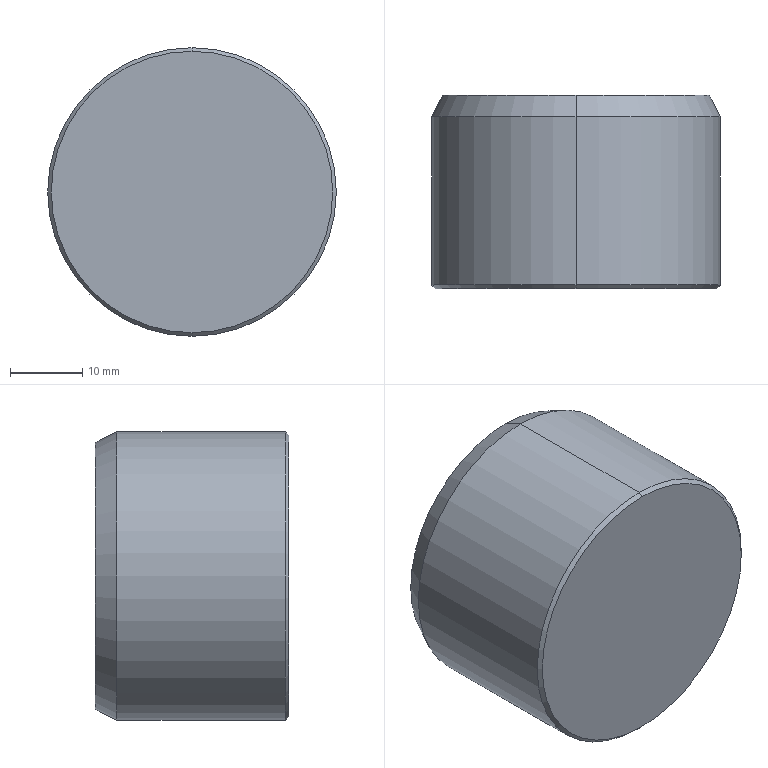Part | SolidWorks | features Chamfer 2, Revolution 1 | 1 solid | 8 faces | box 40 x 26.8 x 40 mm | volume 33387 mm3 | cone 4 | cylinder 2 | plane 2 | commonest cylinder face diameters 40 x2
STEP:
#1=CARTESIAN_POINT('',(0.,-13.4,-19.5));
#2=VERTEX_POINT('',#1);
#3=CARTESIAN_POINT('',(0.,-13.4,19.5));
#4=VERTEX_POINT('',#3);
#5=CARTESIAN_POINT('',(0.,-13.4,0.));
#6=DIRECTION('',(0.,-1.,0.));
#7=DIRECTION('',(0.,0.,-1.));
#8=AXIS2_PLACEMENT_3D('',#5,#6,#7);
#9=CIRCLE('',#8,19.5);
#10=EDGE_CURVE('',#2,#4,#9,.T.);
#11=ORIENTED_EDGE('',*,*,#10,.F.);
#12=CARTESIAN_POINT('',(0.,-12.9,-20.));
#13=VERTEX_POINT('',#12);
#14=CARTESIAN_POINT('',(0.,-13.4,-19.5));
#15=DIRECTION('',(0.,0.7071,-0.7071));
#16=VECTOR('',#15,1000.);
#17=LINE('',#14,#16);
#18=EDGE_CURVE('',#2,#13,#17,.T.);
#19=ORIENTED_EDGE('',*,*,#18,.T.);
#20=CARTESIAN_POINT('',(0.,-12.9,20.));
#21=VERTEX_POINT('',#20);
#22=CARTESIAN_POINT('',(0.,-12.9,0.));
#23=DIRECTION('',(0.,1.,0.));
#24=DIRECTION('',(0.,0.,-1.));
#25=AXIS2_PLACEMENT_3D('',#22,#23,#24);
#26=CIRCLE('',#25,20.);
#27=EDGE_CURVE('',#21,#13,#26,.T.);
#28=ORIENTED_EDGE('',*,*,#27,.F.);
#29=CARTESIAN_POINT('',(0.,-13.4,19.5));
#30=DIRECTION('',(0.,0.7071,0.7071));
#31=VECTOR('',#30,1000.);
#32=LINE('',#29,#31);
#33=EDGE_CURVE('',#4,#21,#32,.T.);
#34=ORIENTED_EDGE('',*,*,#33,.F.);
#35=EDGE_LOOP('',(#11,#19,#28,#34));
#36=FACE_OUTER_BOUND('',#35,.T.);
#37=CARTESIAN_POINT('',(0.,-13.4,0.));
#38=DIRECTION('',(0.,1.,0.));
#39=DIRECTION('',(0.,0.,1.));
#40=AXIS2_PLACEMENT_3D('',#37,#38,#39);
#41=CONICAL_SURFACE('',#40,19.5,0.7854);
#42=ADVANCED_FACE('',(#36),#41,.T.);
#43=CARTESIAN_POINT('',(0.,13.4,18.5));
#44=VERTEX_POINT('',#43);
#45=CARTESIAN_POINT('',(0.,13.4,-18.5));
#46=VERTEX_POINT('',#45);
#47=CARTESIAN_POINT('',(0.,13.4,0.));
#48=DIRECTION('',(0.,1.,0.));
#49=DIRECTION('',(0.,0.,1.));
#50=AXIS2_PLACEMENT_3D('',#47,#48,#49);
#51=CIRCLE('',#50,18.5);
#52=EDGE_CURVE('',#44,#46,#51,.T.);
#53=ORIENTED_EDGE('',*,*,#52,.F.);
#54=CARTESIAN_POINT('',(0.,10.4,20.));
#55=VERTEX_POINT('',#54);
#56=CARTESIAN_POINT('',(0.,10.4,20.));
#57=DIRECTION('',(0.,-0.8944,0.4472));
#58=VECTOR('',#57,1000.);
#59=LINE('',#56,#58);
#60=EDGE_CURVE('',#44,#55,#59,.T.);
#61=ORIENTED_EDGE('',*,*,#60,.T.);
#62=CARTESIAN_POINT('',(0.,10.4,-20.));
#63=VERTEX_POINT('',#62);
#64=CARTESIAN_POINT('',(0.,10.4,0.));
#65=DIRECTION('',(0.,-1.,0.));
#66=DIRECTION('',(0.,0.,1.));
#67=AXIS2_PLACEMENT_3D('',#64,#65,#66);
#68=CIRCLE('',#67,20.);
#69=EDGE_CURVE('',#63,#55,#68,.T.);
#70=ORIENTED_EDGE('',*,*,#69,.F.);
#71=CARTESIAN_POINT('',(0.,10.4,-20.));
#72=DIRECTION('',(0.,-0.8944,-0.4472));
#73=VECTOR('',#72,1000.);
#74=LINE('',#71,#73);
#75=EDGE_CURVE('',#46,#63,#74,.T.);
#76=ORIENTED_EDGE('',*,*,#75,.F.);
#77=EDGE_LOOP('',(#53,#61,#70,#76));
#78=FACE_OUTER_BOUND('',#77,.T.);
#79=CARTESIAN_POINT('',(0.,10.4,0.));
#80=DIRECTION('',(0.,-1.,0.));
#81=DIRECTION('',(0.,0.,-1.));
#82=AXIS2_PLACEMENT_3D('',#79,#80,#81);
#83=CONICAL_SURFACE('',#82,20.,0.4636);
#84=ADVANCED_FACE('',(#78),#83,.T.);
#85=ORIENTED_EDGE('',*,*,#69,.T.);
#86=CARTESIAN_POINT('',(0.,0.,20.));
#87=DIRECTION('',(0.,-1.,0.));
#88=VECTOR('',#87,1000.);
#89=LINE('',#86,#88);
#90=EDGE_CURVE('',#55,#21,#89,.T.);
#91=ORIENTED_EDGE('',*,*,#90,.T.);
#92=ORIENTED_EDGE('',*,*,#27,.T.);
#93=CARTESIAN_POINT('',(0.,0.,-20.));
#94=DIRECTION('',(0.,-1.,0.));
#95=VECTOR('',#94,1000.);
#96=LINE('',#93,#95);
#97=EDGE_CURVE('',#63,#13,#96,.T.);
#98=ORIENTED_EDGE('',*,*,#97,.F.);
#99=EDGE_LOOP('',(#85,#91,#92,#98));
#100=FACE_OUTER_BOUND('',#99,.T.);
#101=CARTESIAN_POINT('',(0.,0.,0.));
#102=DIRECTION('',(0.,-1.,0.));
#103=DIRECTION('',(0.,0.,-1.));
#104=AXIS2_PLACEMENT_3D('',#101,#102,#103);
#105=CYLINDRICAL_SURFACE('',#104,20.);
#106=ADVANCED_FACE('',(#100),#105,.T.);
#107=CARTESIAN_POINT('',(0.,-13.4,0.));
#108=DIRECTION('',(0.,-1.,0.));
#109=DIRECTION('',(0.,0.,-1.));
#110=AXIS2_PLACEMENT_3D('',#107,#108,#109);
#111=CIRCLE('',#110,19.5);
#112=EDGE_CURVE('',#4,#2,#111,.T.);
#113=ORIENTED_EDGE('',*,*,#112,.T.);
#114=ORIENTED_EDGE('',*,*,#10,.T.);
#115=EDGE_LOOP('',(#113,#114));
#116=FACE_OUTER_BOUND('',#115,.T.);
#117=CARTESIAN_POINT('',(20.,-13.4,0.));
#118=DIRECTION('',(0.,-1.,0.));
#119=DIRECTION('',(0.,0.,-1.));
#120=AXIS2_PLACEMENT_3D('',#117,#118,#119);
#121=PLANE('',#120);
#122=ADVANCED_FACE('',(#116),#121,.T.);
#123=ORIENTED_EDGE('',*,*,#90,.F.);
#124=CARTESIAN_POINT('',(0.,10.4,0.));
#125=DIRECTION('',(0.,-1.,0.));
#126=DIRECTION('',(0.,0.,1.));
#127=AXIS2_PLACEMENT_3D('',#124,#125,#126);
#128=CIRCLE('',#127,20.);
#129=EDGE_CURVE('',#55,#63,#128,.T.);
#130=ORIENTED_EDGE('',*,*,#129,.T.);
#131=ORIENTED_EDGE('',*,*,#97,.T.);
#132=CARTESIAN_POINT('',(0.,-12.9,0.));
#133=DIRECTION('',(0.,1.,0.));
#134=DIRECTION('',(0.,0.,-1.));
#135=AXIS2_PLACEMENT_3D('',#132,#133,#134);
#136=CIRCLE('',#135,20.);
#137=EDGE_CURVE('',#13,#21,#136,.T.);
#138=ORIENTED_EDGE('',*,*,#137,.T.);
#139=EDGE_LOOP('',(#123,#130,#131,#138));
#140=FACE_OUTER_BOUND('',#139,.T.);
#141=CARTESIAN_POINT('',(0.,0.,0.));
#142=DIRECTION('',(0.,-1.,0.));
#143=DIRECTION('',(0.,0.,-1.));
#144=AXIS2_PLACEMENT_3D('',#141,#142,#143);
#145=CYLINDRICAL_SURFACE('',#144,20.);
#146=ADVANCED_FACE('',(#140),#145,.T.);
#147=CARTESIAN_POINT('',(0.,13.4,0.));
#148=DIRECTION('',(0.,1.,0.));
#149=DIRECTION('',(0.,0.,1.));
#150=AXIS2_PLACEMENT_3D('',#147,#148,#149);
#151=CIRCLE('',#150,18.5);
#152=EDGE_CURVE('',#46,#44,#151,.T.);
#153=ORIENTED_EDGE('',*,*,#152,.T.);
#154=ORIENTED_EDGE('',*,*,#52,.T.);
#155=EDGE_LOOP('',(#153,#154));
#156=FACE_OUTER_BOUND('',#155,.T.);
#157=CARTESIAN_POINT('',(20.,13.4,0.));
#158=DIRECTION('',(0.,1.,0.));
#159=DIRECTION('',(0.,0.,1.));
#160=AXIS2_PLACEMENT_3D('',#157,#158,#159);
#161=PLANE('',#160);
#162=ADVANCED_FACE('',(#156),#161,.T.);
#163=ORIENTED_EDGE('',*,*,#60,.F.);
#164=ORIENTED_EDGE('',*,*,#152,.F.);
#165=ORIENTED_EDGE('',*,*,#75,.T.);
#166=ORIENTED_EDGE('',*,*,#129,.F.);
#167=EDGE_LOOP('',(#163,#164,#165,#166));
#168=FACE_OUTER_BOUND('',#167,.T.);
#169=CARTESIAN_POINT('',(0.,10.4,0.));
#170=DIRECTION('',(0.,-1.,0.));
#171=DIRECTION('',(0.,0.,-1.));
#172=AXIS2_PLACEMENT_3D('',#169,#170,#171);
#173=CONICAL_SURFACE('',#172,20.,0.4636);
#174=ADVANCED_FACE('',(#168),#173,.T.);
#175=ORIENTED_EDGE('',*,*,#18,.F.);
#176=ORIENTED_EDGE('',*,*,#112,.F.);
#177=ORIENTED_EDGE('',*,*,#33,.T.);
#178=ORIENTED_EDGE('',*,*,#137,.F.);
#179=EDGE_LOOP('',(#175,#176,#177,#178));
#180=FACE_OUTER_BOUND('',#179,.T.);
#181=CARTESIAN_POINT('',(0.,-13.4,0.));
#182=DIRECTION('',(0.,1.,0.));
#183=DIRECTION('',(0.,0.,1.));
#184=AXIS2_PLACEMENT_3D('',#181,#182,#183);
#185=CONICAL_SURFACE('',#184,19.5,0.7854);
#186=ADVANCED_FACE('',(#180),#185,.T.);
#187=CLOSED_SHELL('',(#42,#84,#106,#122,#146,#162,#174,#186));
#188=MANIFOLD_SOLID_BREP('',#187);
#189=CARTESIAN_POINT('',(0.,0.,0.));
#190=DIRECTION('',(0.,0.,1.));
#191=DIRECTION('',(1.,0.,0.));
#192=AXIS2_PLACEMENT_3D('',#189,#190,#191);
#193=(LENGTH_UNIT()NAMED_UNIT(*)SI_UNIT(.MILLI.,.METRE.));
#194=UNCERTAINTY_MEASURE_WITH_UNIT(LENGTH_MEASURE(0.00001),#193,'','');
#195=(NAMED_UNIT(*)PLANE_ANGLE_UNIT()SI_UNIT($,.RADIAN.));
#196=(NAMED_UNIT(*)SI_UNIT($,.STERADIAN.)SOLID_ANGLE_UNIT());
#197=(GEOMETRIC_REPRESENTATION_CONTEXT(3)GLOBAL_UNCERTAINTY_ASSIGNED_CONTEXT((#194))GLOBAL_UNIT_ASSIGNED_CONTEXT((#193,#195,#196))REPRESENTATION_CONTEXT('',''));
#198=ADVANCED_BREP_SHAPE_REPRESENTATION('',(#188,#192),#197);